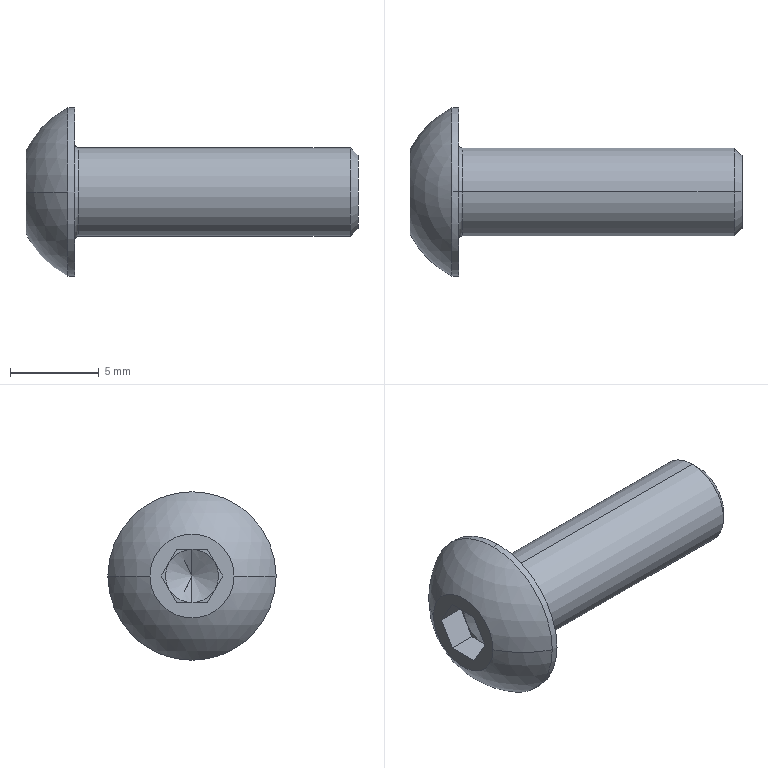Part | STEP file | socket button head screw_iso_ISO 7380 - M5 x 16 - 16N | 1 solid | 27 faces | box 18.75 x 9.5 x 9.5 mm | volume 437.534 mm3 | plane 15 | cone 4 | cylinder 4 | torus 2 | sphere 2 | commonest cylinder face diameters 5 x2 9.5 x2
STEP:
#1=CARTESIAN_POINT('',(2.426,0.,0.));
#2=VERTEX_POINT('',#1);
#3=CARTESIAN_POINT('',(1.56,0.,1.5));
#4=VERTEX_POINT('',#3);
#5=CARTESIAN_POINT('',(2.426,0.,0.));
#6=DIRECTION('',(-0.5,0.,0.866));
#7=VECTOR('',#6,1000.);
#8=LINE('',#5,#7);
#9=EDGE_CURVE('',#2,#4,#8,.T.);
#10=ORIENTED_EDGE('',*,*,#9,.F.);
#11=CARTESIAN_POINT('',(1.56,0.,-1.5));
#12=VERTEX_POINT('',#11);
#13=CARTESIAN_POINT('',(2.426,0.,0.));
#14=DIRECTION('',(-0.5,0.,-0.866));
#15=VECTOR('',#14,1000.);
#16=LINE('',#13,#15);
#17=EDGE_CURVE('',#2,#12,#16,.T.);
#18=ORIENTED_EDGE('',*,*,#17,.T.);
#19=CARTESIAN_POINT('',(1.56,-1.299,-0.75));
#20=VERTEX_POINT('',#19);
#21=CARTESIAN_POINT('',(1.56,0.,0.));
#22=DIRECTION('',(-1.,0.,0.));
#23=DIRECTION('',(0.,0.,1.));
#24=AXIS2_PLACEMENT_3D('',#21,#22,#23);
#25=CIRCLE('',#24,1.5);
#26=EDGE_CURVE('',#12,#20,#25,.T.);
#27=ORIENTED_EDGE('',*,*,#26,.T.);
#28=CARTESIAN_POINT('',(1.56,-1.299,0.75));
#29=VERTEX_POINT('',#28);
#30=CARTESIAN_POINT('',(1.56,0.,0.));
#31=DIRECTION('',(-1.,0.,0.));
#32=DIRECTION('',(0.,0.,1.));
#33=AXIS2_PLACEMENT_3D('',#30,#31,#32);
#34=CIRCLE('',#33,1.5);
#35=EDGE_CURVE('',#20,#29,#34,.T.);
#36=ORIENTED_EDGE('',*,*,#35,.T.);
#37=CARTESIAN_POINT('',(1.56,0.,0.));
#38=DIRECTION('',(-1.,0.,0.));
#39=DIRECTION('',(0.,0.,1.));
#40=AXIS2_PLACEMENT_3D('',#37,#38,#39);
#41=CIRCLE('',#40,1.5);
#42=EDGE_CURVE('',#29,#4,#41,.T.);
#43=ORIENTED_EDGE('',*,*,#42,.T.);
#44=EDGE_LOOP('',(#10,#18,#27,#36,#43));
#45=FACE_OUTER_BOUND('',#44,.T.);
#46=CARTESIAN_POINT('',(-997.574,0.,0.));
#47=DIRECTION('',(-1.,0.,0.));
#48=DIRECTION('',(0.,0.,1.));
#49=AXIS2_PLACEMENT_3D('',#46,#47,#48);
#50=CONICAL_SURFACE('',#49,1732.051,1.047);
#51=ADVANCED_FACE('',(#45),#50,.F.);
#52=CARTESIAN_POINT('',(2.75,0.,-2.7));
#53=VERTEX_POINT('',#52);
#54=CARTESIAN_POINT('',(2.75,0.,2.7));
#55=VERTEX_POINT('',#54);
#56=CARTESIAN_POINT('',(2.75,0.,0.));
#57=DIRECTION('',(-1.,0.,0.));
#58=DIRECTION('',(0.,0.,1.));
#59=AXIS2_PLACEMENT_3D('',#56,#57,#58);
#60=CIRCLE('',#59,2.7);
#61=EDGE_CURVE('',#53,#55,#60,.T.);
#62=ORIENTED_EDGE('',*,*,#61,.F.);
#63=CARTESIAN_POINT('',(2.95,0.,-2.5));
#64=VERTEX_POINT('',#63);
#65=CARTESIAN_POINT('',(2.95,0.,-2.7));
#66=DIRECTION('',(0.,1.,0.));
#67=DIRECTION('',(0.,0.,1.));
#68=AXIS2_PLACEMENT_3D('',#65,#66,#67);
#69=CIRCLE('',#68,0.2);
#70=EDGE_CURVE('',#53,#64,#69,.T.);
#71=ORIENTED_EDGE('',*,*,#70,.T.);
#72=CARTESIAN_POINT('',(2.95,0.,2.5));
#73=VERTEX_POINT('',#72);
#74=CARTESIAN_POINT('',(2.95,0.,0.));
#75=DIRECTION('',(1.,0.,0.));
#76=DIRECTION('',(0.,0.,1.));
#77=AXIS2_PLACEMENT_3D('',#74,#75,#76);
#78=CIRCLE('',#77,2.5);
#79=EDGE_CURVE('',#73,#64,#78,.T.);
#80=ORIENTED_EDGE('',*,*,#79,.F.);
#81=CARTESIAN_POINT('',(2.95,0.,2.7));
#82=DIRECTION('',(0.,-1.,0.));
#83=DIRECTION('',(0.,0.,-1.));
#84=AXIS2_PLACEMENT_3D('',#81,#82,#83);
#85=CIRCLE('',#84,0.2);
#86=EDGE_CURVE('',#55,#73,#85,.T.);
#87=ORIENTED_EDGE('',*,*,#86,.F.);
#88=EDGE_LOOP('',(#62,#71,#80,#87));
#89=FACE_OUTER_BOUND('',#88,.T.);
#90=CARTESIAN_POINT('',(2.95,0.,0.));
#91=DIRECTION('',(-1.,0.,0.));
#92=DIRECTION('',(0.,0.,1.));
#93=AXIS2_PLACEMENT_3D('',#90,#91,#92);
#94=TOROIDAL_SURFACE('',#93,2.7,0.2);
#95=ADVANCED_FACE('',(#89),#94,.F.);
#96=CARTESIAN_POINT('',(18.75,0.,2.055));
#97=VERTEX_POINT('',#96);
#98=CARTESIAN_POINT('',(18.75,0.,-2.055));
#99=VERTEX_POINT('',#98);
#100=CARTESIAN_POINT('',(18.75,0.,0.));
#101=DIRECTION('',(-1.,0.,0.));
#102=DIRECTION('',(0.,0.,1.));
#103=AXIS2_PLACEMENT_3D('',#100,#101,#102);
#104=CIRCLE('',#103,2.055);
#105=EDGE_CURVE('',#97,#99,#104,.T.);
#106=ORIENTED_EDGE('',*,*,#105,.T.);
#107=CARTESIAN_POINT('',(18.305,0.,-2.5));
#108=VERTEX_POINT('',#107);
#109=CARTESIAN_POINT('',(18.75,0.,-2.055));
#110=DIRECTION('',(-0.7071,0.,-0.7071));
#111=VECTOR('',#110,1000.);
#112=LINE('',#109,#111);
#113=EDGE_CURVE('',#99,#108,#112,.T.);
#114=ORIENTED_EDGE('',*,*,#113,.T.);
#115=CARTESIAN_POINT('',(18.305,0.,2.5));
#116=VERTEX_POINT('',#115);
#117=CARTESIAN_POINT('',(18.305,0.,0.));
#118=DIRECTION('',(-1.,0.,0.));
#119=DIRECTION('',(0.,0.,1.));
#120=AXIS2_PLACEMENT_3D('',#117,#118,#119);
#121=CIRCLE('',#120,2.5);
#122=EDGE_CURVE('',#116,#108,#121,.T.);
#123=ORIENTED_EDGE('',*,*,#122,.F.);
#124=CARTESIAN_POINT('',(18.75,0.,2.055));
#125=DIRECTION('',(-0.7071,0.,0.7071));
#126=VECTOR('',#125,1000.);
#127=LINE('',#124,#126);
#128=EDGE_CURVE('',#97,#116,#127,.T.);
#129=ORIENTED_EDGE('',*,*,#128,.F.);
#130=EDGE_LOOP('',(#106,#114,#123,#129));
#131=FACE_OUTER_BOUND('',#130,.T.);
#132=CARTESIAN_POINT('',(18.75,0.,0.));
#133=DIRECTION('',(-1.,0.,0.));
#134=DIRECTION('',(0.,0.,1.));
#135=AXIS2_PLACEMENT_3D('',#132,#133,#134);
#136=CONICAL_SURFACE('',#135,2.055,0.7854);
#137=ADVANCED_FACE('',(#131),#136,.T.);
#138=ORIENTED_EDGE('',*,*,#122,.T.);
#139=CARTESIAN_POINT('',(0.,0.,-2.5));
#140=DIRECTION('',(-1.,0.,0.));
#141=VECTOR('',#140,1000.);
#142=LINE('',#139,#141);
#143=EDGE_CURVE('',#108,#64,#142,.T.);
#144=ORIENTED_EDGE('',*,*,#143,.T.);
#145=CARTESIAN_POINT('',(2.95,0.,0.));
#146=DIRECTION('',(1.,0.,0.));
#147=DIRECTION('',(0.,0.,1.));
#148=AXIS2_PLACEMENT_3D('',#145,#146,#147);
#149=CIRCLE('',#148,2.5);
#150=EDGE_CURVE('',#64,#73,#149,.T.);
#151=ORIENTED_EDGE('',*,*,#150,.T.);
#152=CARTESIAN_POINT('',(0.,0.,2.5));
#153=DIRECTION('',(-1.,0.,0.));
#154=VECTOR('',#153,1000.);
#155=LINE('',#152,#154);
#156=EDGE_CURVE('',#116,#73,#155,.T.);
#157=ORIENTED_EDGE('',*,*,#156,.F.);
#158=EDGE_LOOP('',(#138,#144,#151,#157));
#159=FACE_OUTER_BOUND('',#158,.T.);
#160=CARTESIAN_POINT('',(0.,0.,0.));
#161=DIRECTION('',(-1.,0.,0.));
#162=DIRECTION('',(0.,0.,1.));
#163=AXIS2_PLACEMENT_3D('',#160,#161,#162);
#164=CYLINDRICAL_SURFACE('',#163,2.5);
#165=ADVANCED_FACE('',(#159),#164,.T.);
#166=CARTESIAN_POINT('',(2.75,0.,4.75));
#167=VERTEX_POINT('',#166);
#168=CARTESIAN_POINT('',(2.75,0.,-4.75));
#169=VERTEX_POINT('',#168);
#170=CARTESIAN_POINT('',(2.75,0.,0.));
#171=DIRECTION('',(-1.,0.,0.));
#172=DIRECTION('',(0.,0.,1.));
#173=AXIS2_PLACEMENT_3D('',#170,#171,#172);
#174=CIRCLE('',#173,4.75);
#175=EDGE_CURVE('',#167,#169,#174,.T.);
#176=ORIENTED_EDGE('',*,*,#175,.T.);
#177=CARTESIAN_POINT('',(2.37,0.,-4.75));
#178=VERTEX_POINT('',#177);
#179=CARTESIAN_POINT('',(0.,0.,-4.75));
#180=DIRECTION('',(-1.,0.,0.));
#181=VECTOR('',#180,1000.);
#182=LINE('',#179,#181);
#183=EDGE_CURVE('',#169,#178,#182,.T.);
#184=ORIENTED_EDGE('',*,*,#183,.T.);
#185=CARTESIAN_POINT('',(2.37,4.75,0.));
#186=VERTEX_POINT('',#185);
#187=CARTESIAN_POINT('',(2.37,0.,0.));
#188=DIRECTION('',(-1.,0.,0.));
#189=DIRECTION('',(0.,0.,1.));
#190=AXIS2_PLACEMENT_3D('',#187,#188,#189);
#191=CIRCLE('',#190,4.75);
#192=EDGE_CURVE('',#186,#178,#191,.T.);
#193=ORIENTED_EDGE('',*,*,#192,.F.);
#194=CARTESIAN_POINT('',(2.37,0.,4.75));
#195=VERTEX_POINT('',#194);
#196=CARTESIAN_POINT('',(2.37,0.,0.));
#197=DIRECTION('',(-1.,0.,0.));
#198=DIRECTION('',(0.,0.,1.));
#199=AXIS2_PLACEMENT_3D('',#196,#197,#198);
#200=CIRCLE('',#199,4.75);
#201=EDGE_CURVE('',#195,#186,#200,.T.);
#202=ORIENTED_EDGE('',*,*,#201,.F.);
#203=CARTESIAN_POINT('',(0.,0.,4.75));
#204=DIRECTION('',(-1.,0.,0.));
#205=VECTOR('',#204,1000.);
#206=LINE('',#203,#205);
#207=EDGE_CURVE('',#167,#195,#206,.T.);
#208=ORIENTED_EDGE('',*,*,#207,.F.);
#209=EDGE_LOOP('',(#176,#184,#193,#202,#208));
#210=FACE_OUTER_BOUND('',#209,.T.);
#211=CARTESIAN_POINT('',(0.,0.,0.));
#212=DIRECTION('',(-1.,0.,0.));
#213=DIRECTION('',(0.,0.,1.));
#214=AXIS2_PLACEMENT_3D('',#211,#212,#213);
#215=CYLINDRICAL_SURFACE('',#214,4.75);
#216=ADVANCED_FACE('',(#210),#215,.T.);
#217=ORIENTED_EDGE('',*,*,#192,.T.);
#218=CARTESIAN_POINT('',(2.37,-4.75,0.));
#219=VERTEX_POINT('',#218);
#220=CARTESIAN_POINT('',(2.37,0.,0.));
#221=DIRECTION('',(-1.,0.,0.));
#222=DIRECTION('',(0.,0.,1.));
#223=AXIS2_PLACEMENT_3D('',#220,#221,#222);
#224=CIRCLE('',#223,4.75);
#225=EDGE_CURVE('',#178,#219,#224,.T.);
#226=ORIENTED_EDGE('',*,*,#225,.T.);
#227=CARTESIAN_POINT('',(0.,-2.375,0.));
#228=VERTEX_POINT('',#227);
#229=CARTESIAN_POINT('',(4.755,0.,0.));
#230=DIRECTION('',(0.,0.,-1.));
#231=DIRECTION('',(0.,1.,0.));
#232=AXIS2_PLACEMENT_3D('',#229,#230,#231);
#233=CIRCLE('',#232,5.315);
#234=EDGE_CURVE('',#219,#228,#233,.T.);
#235=ORIENTED_EDGE('',*,*,#234,.T.);
#236=CARTESIAN_POINT('',(0.,2.375,0.));
#237=VERTEX_POINT('',#236);
#238=CARTESIAN_POINT('',(0.,0.,0.));
#239=DIRECTION('',(-1.,0.,0.));
#240=DIRECTION('',(0.,0.,1.));
#241=AXIS2_PLACEMENT_3D('',#238,#239,#240);
#242=CIRCLE('',#241,2.375);
#243=EDGE_CURVE('',#237,#228,#242,.T.);
#244=ORIENTED_EDGE('',*,*,#243,.F.);
#245=CARTESIAN_POINT('',(4.755,0.,0.));
#246=DIRECTION('',(0.,0.,1.));
#247=DIRECTION('',(1.,0.,0.));
#248=AXIS2_PLACEMENT_3D('',#245,#246,#247);
#249=CIRCLE('',#248,5.315);
#250=EDGE_CURVE('',#186,#237,#249,.T.);
#251=ORIENTED_EDGE('',*,*,#250,.F.);
#252=EDGE_LOOP('',(#217,#226,#235,#244,#251));
#253=FACE_OUTER_BOUND('',#252,.T.);
#254=CARTESIAN_POINT('',(4.755,0.,0.));
#255=DIRECTION('',(0.,0.,-1.));
#256=DIRECTION('',(0.,1.,0.));
#257=AXIS2_PLACEMENT_3D('',#254,#255,#256);
#258=SPHERICAL_SURFACE('',#257,5.315);
#259=ADVANCED_FACE('',(#253),#258,.T.);
#260=ORIENTED_EDGE('',*,*,#243,.T.);
#261=CARTESIAN_POINT('',(0.,0.,0.));
#262=DIRECTION('',(-1.,0.,0.));
#263=DIRECTION('',(0.,0.,1.));
#264=AXIS2_PLACEMENT_3D('',#261,#262,#263);
#265=CIRCLE('',#264,2.375);
#266=EDGE_CURVE('',#228,#237,#265,.T.);
#267=ORIENTED_EDGE('',*,*,#266,.T.);
#268=EDGE_LOOP('',(#260,#267));
#269=FACE_OUTER_BOUND('',#268,.T.);
#270=CARTESIAN_POINT('',(0.,0.866,1.5));
#271=VERTEX_POINT('',#270);
#272=CARTESIAN_POINT('',(0.,-0.866,1.5));
#273=VERTEX_POINT('',#272);
#274=CARTESIAN_POINT('',(0.,-0.866,1.5));
#275=DIRECTION('',(0.,-1.,0.));
#276=VECTOR('',#275,1000.);
#277=LINE('',#274,#276);
#278=EDGE_CURVE('',#271,#273,#277,.T.);
#279=ORIENTED_EDGE('',*,*,#278,.T.);
#280=CARTESIAN_POINT('',(0.,-1.732,0.));
#281=VERTEX_POINT('',#280);
#282=CARTESIAN_POINT('',(0.,-1.732,0.));
#283=DIRECTION('',(0.,-0.5,-0.866));
#284=VECTOR('',#283,1000.);
#285=LINE('',#282,#284);
#286=EDGE_CURVE('',#273,#281,#285,.T.);
#287=ORIENTED_EDGE('',*,*,#286,.T.);
#288=CARTESIAN_POINT('',(0.,-0.866,-1.5));
#289=VERTEX_POINT('',#288);
#290=CARTESIAN_POINT('',(0.,-0.866,-1.5));
#291=DIRECTION('',(0.,0.5,-0.866));
#292=VECTOR('',#291,1000.);
#293=LINE('',#290,#292);
#294=EDGE_CURVE('',#281,#289,#293,.T.);
#295=ORIENTED_EDGE('',*,*,#294,.T.);
#296=CARTESIAN_POINT('',(0.,0.866,-1.5));
#297=VERTEX_POINT('',#296);
#298=CARTESIAN_POINT('',(0.,0.866,-1.5));
#299=DIRECTION('',(0.,1.,0.));
#300=VECTOR('',#299,1000.);
#301=LINE('',#298,#300);
#302=EDGE_CURVE('',#289,#297,#301,.T.);
#303=ORIENTED_EDGE('',*,*,#302,.T.);
#304=CARTESIAN_POINT('',(0.,1.732,0.));
#305=VERTEX_POINT('',#304);
#306=CARTESIAN_POINT('',(0.,1.732,0.));
#307=DIRECTION('',(0.,0.5,0.866));
#308=VECTOR('',#307,1000.);
#309=LINE('',#306,#308);
#310=EDGE_CURVE('',#297,#305,#309,.T.);
#311=ORIENTED_EDGE('',*,*,#310,.T.);
#312=CARTESIAN_POINT('',(0.,0.866,1.5));
#313=DIRECTION('',(0.,-0.5,0.866));
#314=VECTOR('',#313,1000.);
#315=LINE('',#312,#314);
#316=EDGE_CURVE('',#305,#271,#315,.T.);
#317=ORIENTED_EDGE('',*,*,#316,.T.);
#318=EDGE_LOOP('',(#279,#287,#295,#303,#311,#317));
#319=FACE_BOUND('',#318,.T.);
#320=CARTESIAN_POINT('',(0.,0.,0.));
#321=DIRECTION('',(-1.,0.,0.));
#322=DIRECTION('',(0.,0.,1.));
#323=AXIS2_PLACEMENT_3D('',#320,#321,#322);
#324=PLANE('',#323);
#325=ADVANCED_FACE('',(#269,#319),#324,.T.);
#326=ORIENTED_EDGE('',*,*,#234,.F.);
#327=CARTESIAN_POINT('',(2.37,0.,0.));
#328=DIRECTION('',(-1.,0.,0.));
#329=DIRECTION('',(0.,0.,1.));
#330=AXIS2_PLACEMENT_3D('',#327,#328,#329);
#331=CIRCLE('',#330,4.75);
#332=EDGE_CURVE('',#219,#195,#331,.T.);
#333=ORIENTED_EDGE('',*,*,#332,.T.);
#334=ORIENTED_EDGE('',*,*,#201,.T.);
#335=ORIENTED_EDGE('',*,*,#250,.T.);
#336=ORIENTED_EDGE('',*,*,#266,.F.);
#337=EDGE_LOOP('',(#326,#333,#334,#335,#336));
#338=FACE_OUTER_BOUND('',#337,.T.);
#339=CARTESIAN_POINT('',(4.755,0.,0.));
#340=DIRECTION('',(0.,0.,-1.));
#341=DIRECTION('',(0.,1.,0.));
#342=AXIS2_PLACEMENT_3D('',#339,#340,#341);
#343=SPHERICAL_SURFACE('',#342,5.315);
#344=ADVANCED_FACE('',(#338),#343,.T.);
#345=ORIENTED_EDGE('',*,*,#183,.F.);
#346=CARTESIAN_POINT('',(2.75,0.,0.));
#347=DIRECTION('',(-1.,0.,0.));
#348=DIRECTION('',(0.,0.,1.));
#349=AXIS2_PLACEMENT_3D('',#346,#347,#348);
#350=CIRCLE('',#349,4.75);
#351=EDGE_CURVE('',#169,#167,#350,.T.);
#352=ORIENTED_EDGE('',*,*,#351,.T.);
#353=ORIENTED_EDGE('',*,*,#207,.T.);
#354=ORIENTED_EDGE('',*,*,#332,.F.);
#355=ORIENTED_EDGE('',*,*,#225,.F.);
#356=EDGE_LOOP('',(#345,#352,#353,#354,#355));
#357=FACE_OUTER_BOUND('',#356,.T.);
#358=CARTESIAN_POINT('',(0.,0.,0.));
#359=DIRECTION('',(-1.,0.,0.));
#360=DIRECTION('',(0.,0.,1.));
#361=AXIS2_PLACEMENT_3D('',#358,#359,#360);
#362=CYLINDRICAL_SURFACE('',#361,4.75);
#363=ADVANCED_FACE('',(#357),#362,.T.);
#364=CARTESIAN_POINT('',(2.75,0.,0.));
#365=DIRECTION('',(-1.,0.,0.));
#366=DIRECTION('',(0.,0.,1.));
#367=AXIS2_PLACEMENT_3D('',#364,#365,#366);
#368=CIRCLE('',#367,2.7);
#369=EDGE_CURVE('',#55,#53,#368,.T.);
#370=ORIENTED_EDGE('',*,*,#369,.T.);
#371=ORIENTED_EDGE('',*,*,#61,.T.);
#372=EDGE_LOOP('',(#370,#371));
#373=FACE_BOUND('',#372,.T.);
#374=ORIENTED_EDGE('',*,*,#175,.F.);
#375=ORIENTED_EDGE('',*,*,#351,.F.);
#376=EDGE_LOOP('',(#374,#375));
#377=FACE_OUTER_BOUND('',#376,.T.);
#378=CARTESIAN_POINT('',(2.75,2.5,0.));
#379=DIRECTION('',(-1.,0.,0.));
#380=DIRECTION('',(0.,0.,1.));
#381=AXIS2_PLACEMENT_3D('',#378,#379,#380);
#382=PLANE('',#381);
#383=ADVANCED_FACE('',(#373,#377),#382,.F.);
#384=ORIENTED_EDGE('',*,*,#143,.F.);
#385=CARTESIAN_POINT('',(18.305,0.,0.));
#386=DIRECTION('',(-1.,0.,0.));
#387=DIRECTION('',(0.,0.,1.));
#388=AXIS2_PLACEMENT_3D('',#385,#386,#387);
#389=CIRCLE('',#388,2.5);
#390=EDGE_CURVE('',#108,#116,#389,.T.);
#391=ORIENTED_EDGE('',*,*,#390,.T.);
#392=ORIENTED_EDGE('',*,*,#156,.T.);
#393=ORIENTED_EDGE('',*,*,#79,.T.);
#394=EDGE_LOOP('',(#384,#391,#392,#393));
#395=FACE_OUTER_BOUND('',#394,.T.);
#396=CARTESIAN_POINT('',(0.,0.,0.));
#397=DIRECTION('',(-1.,0.,0.));
#398=DIRECTION('',(0.,0.,1.));
#399=AXIS2_PLACEMENT_3D('',#396,#397,#398);
#400=CYLINDRICAL_SURFACE('',#399,2.5);
#401=ADVANCED_FACE('',(#395),#400,.T.);
#402=ORIENTED_EDGE('',*,*,#113,.F.);
#403=CARTESIAN_POINT('',(18.75,0.,0.));
#404=DIRECTION('',(-1.,0.,0.));
#405=DIRECTION('',(0.,0.,1.));
#406=AXIS2_PLACEMENT_3D('',#403,#404,#405);
#407=CIRCLE('',#406,2.055);
#408=EDGE_CURVE('',#99,#97,#407,.T.);
#409=ORIENTED_EDGE('',*,*,#408,.T.);
#410=ORIENTED_EDGE('',*,*,#128,.T.);
#411=ORIENTED_EDGE('',*,*,#390,.F.);
#412=EDGE_LOOP('',(#402,#409,#410,#411));
#413=FACE_OUTER_BOUND('',#412,.T.);
#414=CARTESIAN_POINT('',(18.75,0.,0.));
#415=DIRECTION('',(-1.,0.,0.));
#416=DIRECTION('',(0.,0.,1.));
#417=AXIS2_PLACEMENT_3D('',#414,#415,#416);
#418=CONICAL_SURFACE('',#417,2.055,0.7854);
#419=ADVANCED_FACE('',(#413),#418,.T.);
#420=ORIENTED_EDGE('',*,*,#105,.F.);
#421=ORIENTED_EDGE('',*,*,#408,.F.);
#422=EDGE_LOOP('',(#420,#421));
#423=FACE_OUTER_BOUND('',#422,.T.);
#424=CARTESIAN_POINT('',(18.75,0.,0.));
#425=DIRECTION('',(-1.,0.,0.));
#426=DIRECTION('',(0.,0.,1.));
#427=AXIS2_PLACEMENT_3D('',#424,#425,#426);
#428=PLANE('',#427);
#429=ADVANCED_FACE('',(#423),#428,.F.);
#430=ORIENTED_EDGE('',*,*,#70,.F.);
#431=ORIENTED_EDGE('',*,*,#369,.F.);
#432=ORIENTED_EDGE('',*,*,#86,.T.);
#433=ORIENTED_EDGE('',*,*,#150,.F.);
#434=EDGE_LOOP('',(#430,#431,#432,#433));
#435=FACE_OUTER_BOUND('',#434,.T.);
#436=CARTESIAN_POINT('',(2.95,0.,0.));
#437=DIRECTION('',(-1.,0.,0.));
#438=DIRECTION('',(0.,0.,1.));
#439=AXIS2_PLACEMENT_3D('',#436,#437,#438);
#440=TOROIDAL_SURFACE('',#439,2.7,0.2);
#441=ADVANCED_FACE('',(#435),#440,.F.);
#442=CARTESIAN_POINT('',(1.56,-0.866,1.5));
#443=VERTEX_POINT('',#442);
#444=CARTESIAN_POINT('',(1.56,-1.732,0.));
#445=DIRECTION('',(0.,-0.5,-0.866));
#446=VECTOR('',#445,1000.);
#447=LINE('',#444,#446);
#448=EDGE_CURVE('',#443,#29,#447,.T.);
#449=ORIENTED_EDGE('',*,*,#448,.T.);
#450=CARTESIAN_POINT('',(1.56,-1.732,0.));
#451=VERTEX_POINT('',#450);
#452=CARTESIAN_POINT('',(1.56,-1.732,0.));
#453=DIRECTION('',(0.,-0.5,-0.866));
#454=VECTOR('',#453,1000.);
#455=LINE('',#452,#454);
#456=EDGE_CURVE('',#29,#451,#455,.T.);
#457=ORIENTED_EDGE('',*,*,#456,.T.);
#458=CARTESIAN_POINT('',(1.56,-1.732,0.));
#459=DIRECTION('',(-1.,0.,0.));
#460=VECTOR('',#459,1000.);
#461=LINE('',#458,#460);
#462=EDGE_CURVE('',#451,#281,#461,.T.);
#463=ORIENTED_EDGE('',*,*,#462,.T.);
#464=ORIENTED_EDGE('',*,*,#286,.F.);
#465=CARTESIAN_POINT('',(1.56,-0.866,1.5));
#466=DIRECTION('',(-1.,0.,0.));
#467=VECTOR('',#466,1000.);
#468=LINE('',#465,#467);
#469=EDGE_CURVE('',#443,#273,#468,.T.);
#470=ORIENTED_EDGE('',*,*,#469,.F.);
#471=EDGE_LOOP('',(#449,#457,#463,#464,#470));
#472=FACE_OUTER_BOUND('',#471,.T.);
#473=CARTESIAN_POINT('',(1.56,-1.732,0.));
#474=DIRECTION('',(0.,0.866,-0.5));
#475=DIRECTION('',(0.,0.5,0.866));
#476=AXIS2_PLACEMENT_3D('',#473,#474,#475);
#477=PLANE('',#476);
#478=ADVANCED_FACE('',(#472),#477,.T.);
#479=CARTESIAN_POINT('',(1.56,-0.866,-1.5));
#480=DIRECTION('',(0.,0.5,-0.866));
#481=VECTOR('',#480,1000.);
#482=LINE('',#479,#481);
#483=EDGE_CURVE('',#451,#20,#482,.T.);
#484=ORIENTED_EDGE('',*,*,#483,.T.);
#485=CARTESIAN_POINT('',(1.56,-0.866,-1.5));
#486=VERTEX_POINT('',#485);
#487=CARTESIAN_POINT('',(1.56,-0.866,-1.5));
#488=DIRECTION('',(0.,0.5,-0.866));
#489=VECTOR('',#488,1000.);
#490=LINE('',#487,#489);
#491=EDGE_CURVE('',#20,#486,#490,.T.);
#492=ORIENTED_EDGE('',*,*,#491,.T.);
#493=CARTESIAN_POINT('',(1.56,-0.866,-1.5));
#494=DIRECTION('',(-1.,0.,0.));
#495=VECTOR('',#494,1000.);
#496=LINE('',#493,#495);
#497=EDGE_CURVE('',#486,#289,#496,.T.);
#498=ORIENTED_EDGE('',*,*,#497,.T.);
#499=ORIENTED_EDGE('',*,*,#294,.F.);
#500=ORIENTED_EDGE('',*,*,#462,.F.);
#501=EDGE_LOOP('',(#484,#492,#498,#499,#500));
#502=FACE_OUTER_BOUND('',#501,.T.);
#503=CARTESIAN_POINT('',(1.56,-0.866,-1.5));
#504=DIRECTION('',(0.,0.866,0.5));
#505=DIRECTION('',(0.,-0.5,0.866));
#506=AXIS2_PLACEMENT_3D('',#503,#504,#505);
#507=PLANE('',#506);
#508=ADVANCED_FACE('',(#502),#507,.T.);
#509=CARTESIAN_POINT('',(1.56,0.866,-1.5));
#510=DIRECTION('',(0.,1.,0.));
#511=VECTOR('',#510,1000.);
#512=LINE('',#509,#511);
#513=EDGE_CURVE('',#486,#12,#512,.T.);
#514=ORIENTED_EDGE('',*,*,#513,.T.);
#515=CARTESIAN_POINT('',(1.56,0.866,-1.5));
#516=VERTEX_POINT('',#515);
#517=CARTESIAN_POINT('',(1.56,0.866,-1.5));
#518=DIRECTION('',(0.,1.,0.));
#519=VECTOR('',#518,1000.);
#520=LINE('',#517,#519);
#521=EDGE_CURVE('',#12,#516,#520,.T.);
#522=ORIENTED_EDGE('',*,*,#521,.T.);
#523=CARTESIAN_POINT('',(1.56,0.866,-1.5));
#524=DIRECTION('',(-1.,0.,0.));
#525=VECTOR('',#524,1000.);
#526=LINE('',#523,#525);
#527=EDGE_CURVE('',#516,#297,#526,.T.);
#528=ORIENTED_EDGE('',*,*,#527,.T.);
#529=ORIENTED_EDGE('',*,*,#302,.F.);
#530=ORIENTED_EDGE('',*,*,#497,.F.);
#531=EDGE_LOOP('',(#514,#522,#528,#529,#530));
#532=FACE_OUTER_BOUND('',#531,.T.);
#533=CARTESIAN_POINT('',(1.56,0.866,-1.5));
#534=DIRECTION('',(0.,0.,1.));
#535=DIRECTION('',(1.,0.,0.));
#536=AXIS2_PLACEMENT_3D('',#533,#534,#535);
#537=PLANE('',#536);
#538=ADVANCED_FACE('',(#532),#537,.T.);
#539=CARTESIAN_POINT('',(1.56,1.299,-0.75));
#540=VERTEX_POINT('',#539);
#541=CARTESIAN_POINT('',(1.56,1.732,0.));
#542=DIRECTION('',(0.,0.5,0.866));
#543=VECTOR('',#542,1000.);
#544=LINE('',#541,#543);
#545=EDGE_CURVE('',#516,#540,#544,.T.);
#546=ORIENTED_EDGE('',*,*,#545,.T.);
#547=CARTESIAN_POINT('',(1.56,1.732,0.));
#548=VERTEX_POINT('',#547);
#549=CARTESIAN_POINT('',(1.56,1.732,0.));
#550=DIRECTION('',(0.,0.5,0.866));
#551=VECTOR('',#550,1000.);
#552=LINE('',#549,#551);
#553=EDGE_CURVE('',#540,#548,#552,.T.);
#554=ORIENTED_EDGE('',*,*,#553,.T.);
#555=CARTESIAN_POINT('',(1.56,1.732,0.));
#556=DIRECTION('',(-1.,0.,0.));
#557=VECTOR('',#556,1000.);
#558=LINE('',#555,#557);
#559=EDGE_CURVE('',#548,#305,#558,.T.);
#560=ORIENTED_EDGE('',*,*,#559,.T.);
#561=ORIENTED_EDGE('',*,*,#310,.F.);
#562=ORIENTED_EDGE('',*,*,#527,.F.);
#563=EDGE_LOOP('',(#546,#554,#560,#561,#562));
#564=FACE_OUTER_BOUND('',#563,.T.);
#565=CARTESIAN_POINT('',(1.56,1.732,0.));
#566=DIRECTION('',(0.,-0.866,0.5));
#567=DIRECTION('',(0.,-0.5,-0.866));
#568=AXIS2_PLACEMENT_3D('',#565,#566,#567);
#569=PLANE('',#568);
#570=ADVANCED_FACE('',(#564),#569,.T.);
#571=CARTESIAN_POINT('',(1.56,1.299,0.75));
#572=VERTEX_POINT('',#571);
#573=CARTESIAN_POINT('',(1.56,0.866,1.5));
#574=DIRECTION('',(0.,-0.5,0.866));
#575=VECTOR('',#574,1000.);
#576=LINE('',#573,#575);
#577=EDGE_CURVE('',#548,#572,#576,.T.);
#578=ORIENTED_EDGE('',*,*,#577,.T.);
#579=CARTESIAN_POINT('',(1.56,0.866,1.5));
#580=VERTEX_POINT('',#579);
#581=CARTESIAN_POINT('',(1.56,0.866,1.5));
#582=DIRECTION('',(0.,-0.5,0.866));
#583=VECTOR('',#582,1000.);
#584=LINE('',#581,#583);
#585=EDGE_CURVE('',#572,#580,#584,.T.);
#586=ORIENTED_EDGE('',*,*,#585,.T.);
#587=CARTESIAN_POINT('',(1.56,0.866,1.5));
#588=DIRECTION('',(-1.,0.,0.));
#589=VECTOR('',#588,1000.);
#590=LINE('',#587,#589);
#591=EDGE_CURVE('',#580,#271,#590,.T.);
#592=ORIENTED_EDGE('',*,*,#591,.T.);
#593=ORIENTED_EDGE('',*,*,#316,.F.);
#594=ORIENTED_EDGE('',*,*,#559,.F.);
#595=EDGE_LOOP('',(#578,#586,#592,#593,#594));
#596=FACE_OUTER_BOUND('',#595,.T.);
#597=CARTESIAN_POINT('',(1.56,0.866,1.5));
#598=DIRECTION('',(0.,-0.866,-0.5));
#599=DIRECTION('',(0.,0.5,-0.866));
#600=AXIS2_PLACEMENT_3D('',#597,#598,#599);
#601=PLANE('',#600);
#602=ADVANCED_FACE('',(#596),#601,.T.);
#603=CARTESIAN_POINT('',(1.56,-0.866,1.5));
#604=DIRECTION('',(0.,-1.,0.));
#605=VECTOR('',#604,1000.);
#606=LINE('',#603,#605);
#607=EDGE_CURVE('',#580,#4,#606,.T.);
#608=ORIENTED_EDGE('',*,*,#607,.T.);
#609=CARTESIAN_POINT('',(1.56,-0.866,1.5));
#610=DIRECTION('',(0.,-1.,0.));
#611=VECTOR('',#610,1000.);
#612=LINE('',#609,#611);
#613=EDGE_CURVE('',#4,#443,#612,.T.);
#614=ORIENTED_EDGE('',*,*,#613,.T.);
#615=ORIENTED_EDGE('',*,*,#469,.T.);
#616=ORIENTED_EDGE('',*,*,#278,.F.);
#617=ORIENTED_EDGE('',*,*,#591,.F.);
#618=EDGE_LOOP('',(#608,#614,#615,#616,#617));
#619=FACE_OUTER_BOUND('',#618,.T.);
#620=CARTESIAN_POINT('',(1.56,-0.866,1.5));
#621=DIRECTION('',(0.,0.,-1.));
#622=DIRECTION('',(-1.,0.,0.));
#623=AXIS2_PLACEMENT_3D('',#620,#621,#622);
#624=PLANE('',#623);
#625=ADVANCED_FACE('',(#619),#624,.T.);
#626=CARTESIAN_POINT('',(1.56,0.,0.));
#627=DIRECTION('',(-1.,0.,0.));
#628=DIRECTION('',(0.,0.,1.));
#629=AXIS2_PLACEMENT_3D('',#626,#627,#628);
#630=CIRCLE('',#629,1.5);
#631=EDGE_CURVE('',#540,#12,#630,.T.);
#632=ORIENTED_EDGE('',*,*,#631,.F.);
#633=ORIENTED_EDGE('',*,*,#545,.F.);
#634=ORIENTED_EDGE('',*,*,#521,.F.);
#635=EDGE_LOOP('',(#632,#633,#634));
#636=FACE_OUTER_BOUND('',#635,.T.);
#637=CARTESIAN_POINT('',(1.56,-1.732,0.));
#638=DIRECTION('',(1.,0.,0.));
#639=DIRECTION('',(0.,0.,-1.));
#640=AXIS2_PLACEMENT_3D('',#637,#638,#639);
#641=PLANE('',#640);
#642=ADVANCED_FACE('',(#636),#641,.F.);
#643=CARTESIAN_POINT('',(1.56,0.,0.));
#644=DIRECTION('',(-1.,0.,0.));
#645=DIRECTION('',(0.,0.,1.));
#646=AXIS2_PLACEMENT_3D('',#643,#644,#645);
#647=CIRCLE('',#646,1.5);
#648=EDGE_CURVE('',#572,#540,#647,.T.);
#649=ORIENTED_EDGE('',*,*,#648,.F.);
#650=ORIENTED_EDGE('',*,*,#577,.F.);
#651=ORIENTED_EDGE('',*,*,#553,.F.);
#652=EDGE_LOOP('',(#649,#650,#651));
#653=FACE_OUTER_BOUND('',#652,.T.);
#654=CARTESIAN_POINT('',(1.56,-1.732,0.));
#655=DIRECTION('',(1.,0.,0.));
#656=DIRECTION('',(0.,0.,-1.));
#657=AXIS2_PLACEMENT_3D('',#654,#655,#656);
#658=PLANE('',#657);
#659=ADVANCED_FACE('',(#653),#658,.F.);
#660=CARTESIAN_POINT('',(1.56,0.,0.));
#661=DIRECTION('',(-1.,0.,0.));
#662=DIRECTION('',(0.,0.,1.));
#663=AXIS2_PLACEMENT_3D('',#660,#661,#662);
#664=CIRCLE('',#663,1.5);
#665=EDGE_CURVE('',#4,#572,#664,.T.);
#666=ORIENTED_EDGE('',*,*,#665,.F.);
#667=ORIENTED_EDGE('',*,*,#607,.F.);
#668=ORIENTED_EDGE('',*,*,#585,.F.);
#669=EDGE_LOOP('',(#666,#667,#668));
#670=FACE_OUTER_BOUND('',#669,.T.);
#671=CARTESIAN_POINT('',(1.56,-1.732,0.));
#672=DIRECTION('',(1.,0.,0.));
#673=DIRECTION('',(0.,0.,-1.));
#674=AXIS2_PLACEMENT_3D('',#671,#672,#673);
#675=PLANE('',#674);
#676=ADVANCED_FACE('',(#670),#675,.F.);
#677=ORIENTED_EDGE('',*,*,#42,.F.);
#678=ORIENTED_EDGE('',*,*,#448,.F.);
#679=ORIENTED_EDGE('',*,*,#613,.F.);
#680=EDGE_LOOP('',(#677,#678,#679));
#681=FACE_OUTER_BOUND('',#680,.T.);
#682=CARTESIAN_POINT('',(1.56,-1.732,0.));
#683=DIRECTION('',(1.,0.,0.));
#684=DIRECTION('',(0.,0.,-1.));
#685=AXIS2_PLACEMENT_3D('',#682,#683,#684);
#686=PLANE('',#685);
#687=ADVANCED_FACE('',(#681),#686,.F.);
#688=ORIENTED_EDGE('',*,*,#35,.F.);
#689=ORIENTED_EDGE('',*,*,#483,.F.);
#690=ORIENTED_EDGE('',*,*,#456,.F.);
#691=EDGE_LOOP('',(#688,#689,#690));
#692=FACE_OUTER_BOUND('',#691,.T.);
#693=CARTESIAN_POINT('',(1.56,-1.732,0.));
#694=DIRECTION('',(1.,0.,0.));
#695=DIRECTION('',(0.,0.,-1.));
#696=AXIS2_PLACEMENT_3D('',#693,#694,#695);
#697=PLANE('',#696);
#698=ADVANCED_FACE('',(#692),#697,.F.);
#699=ORIENTED_EDGE('',*,*,#26,.F.);
#700=ORIENTED_EDGE('',*,*,#513,.F.);
#701=ORIENTED_EDGE('',*,*,#491,.F.);
#702=EDGE_LOOP('',(#699,#700,#701));
#703=FACE_OUTER_BOUND('',#702,.T.);
#704=CARTESIAN_POINT('',(1.56,-1.732,0.));
#705=DIRECTION('',(1.,0.,0.));
#706=DIRECTION('',(0.,0.,-1.));
#707=AXIS2_PLACEMENT_3D('',#704,#705,#706);
#708=PLANE('',#707);
#709=ADVANCED_FACE('',(#703),#708,.F.);
#710=ORIENTED_EDGE('',*,*,#17,.F.);
#711=ORIENTED_EDGE('',*,*,#9,.T.);
#712=ORIENTED_EDGE('',*,*,#665,.T.);
#713=ORIENTED_EDGE('',*,*,#648,.T.);
#714=ORIENTED_EDGE('',*,*,#631,.T.);
#715=EDGE_LOOP('',(#710,#711,#712,#713,#714));
#716=FACE_OUTER_BOUND('',#715,.T.);
#717=CARTESIAN_POINT('',(-997.574,0.,0.));
#718=DIRECTION('',(-1.,0.,0.));
#719=DIRECTION('',(0.,0.,1.));
#720=AXIS2_PLACEMENT_3D('',#717,#718,#719);
#721=CONICAL_SURFACE('',#720,1732.051,1.047);
#722=ADVANCED_FACE('',(#716),#721,.F.);
#723=CLOSED_SHELL('',(#51,#95,#137,#165,#216,#259,#325,#344,#363,#383,#401,#419,#429,#441,#478,#508,#538,#570,#602,#625,#642,#659,#676,#687,#698,#709,#722));
#724=MANIFOLD_SOLID_BREP('',#723);
#725=CARTESIAN_POINT('',(0.,0.,0.));
#726=DIRECTION('',(0.,0.,1.));
#727=DIRECTION('',(1.,0.,0.));
#728=AXIS2_PLACEMENT_3D('',#725,#726,#727);
#729=(LENGTH_UNIT()NAMED_UNIT(*)SI_UNIT(.MILLI.,.METRE.));
#730=UNCERTAINTY_MEASURE_WITH_UNIT(LENGTH_MEASURE(0.00001),#729,'','');
#731=(NAMED_UNIT(*)PLANE_ANGLE_UNIT()SI_UNIT($,.RADIAN.));
#732=(NAMED_UNIT(*)SI_UNIT($,.STERADIAN.)SOLID_ANGLE_UNIT());
#733=(GEOMETRIC_REPRESENTATION_CONTEXT(3)GLOBAL_UNCERTAINTY_ASSIGNED_CONTEXT((#730))GLOBAL_UNIT_ASSIGNED_CONTEXT((#729,#731,#732))REPRESENTATION_CONTEXT('',''));
#734=ADVANCED_BREP_SHAPE_REPRESENTATION('',(#724,#728),#733);